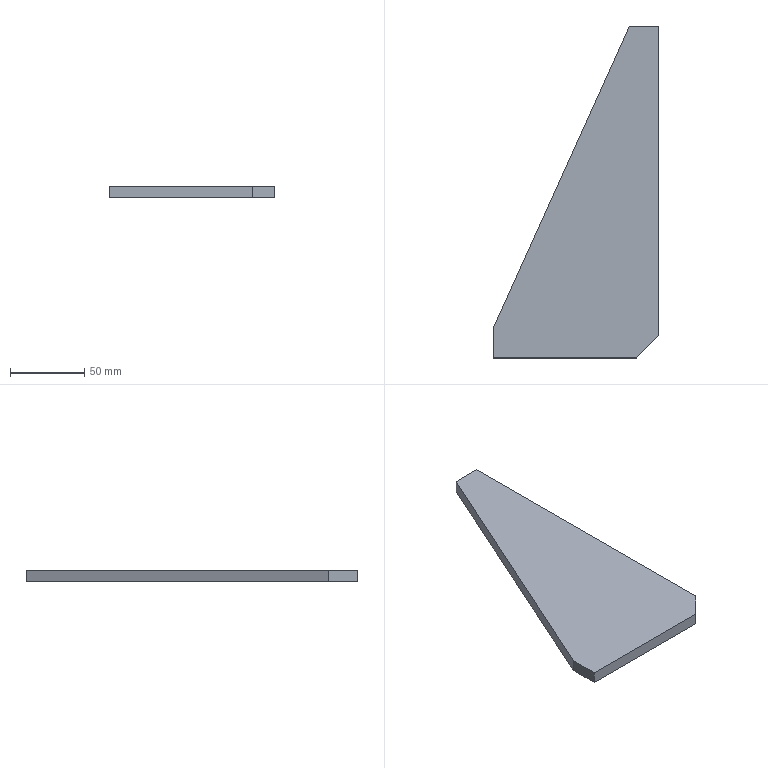Part | STEP file | 02-Rib plate 1 | 1 solid | 8 faces | box 112 x 224 x 8 mm | volume 124732 mm3 | plane 8
STEP:
#1=CARTESIAN_POINT('',(0.,0.,0.));
#2=DIRECTION('',(0.,0.,1.));
#3=DIRECTION('',(1.,0.,0.));
#4=AXIS2_PLACEMENT_3D('',#1,#2,#3);
#5=CARTESIAN_POINT('',(0.,-209.,0.));
#6=VERTEX_POINT('',#5);
#7=CARTESIAN_POINT('',(0.,0.,0.));
#8=VERTEX_POINT('',#7);
#9=CARTESIAN_POINT('',(0.,0.,0.));
#10=DIRECTION('',(0.,1.,0.));
#11=VECTOR('',#10,1.);
#12=LINE('',#9,#11);
#13=CARTESIAN_POINT('',(0.,0.,8.));
#14=DIRECTION('',(-1.,0.,0.));
#15=DIRECTION('',(0.,-1.,0.));
#16=AXIS2_PLACEMENT_3D('',#13,#14,#15);
#17=PLANE('',#16);
#18=CARTESIAN_POINT('',(0.,-8.));
#19=DIRECTION('',(-1.,0.));
#20=VECTOR('',#19,1.);
#21=LINE('',#18,#20);
#22=(GEOMETRIC_REPRESENTATION_CONTEXT(2)PARAMETRIC_REPRESENTATION_CONTEXT()REPRESENTATION_CONTEXT('',''));
#23=DEFINITIONAL_REPRESENTATION('',(#21),#22);
#24=PCURVE('',#17,#23);
#25=CARTESIAN_POINT('',(0.,0.,0.));
#26=DIRECTION('',(0.,0.,-1.));
#27=DIRECTION('',(-1.,0.,0.));
#28=AXIS2_PLACEMENT_3D('',#25,#26,#27);
#29=PLANE('',#28);
#30=CARTESIAN_POINT('',(0.,0.));
#31=DIRECTION('',(0.,1.));
#32=VECTOR('',#31,1.);
#33=LINE('',#30,#32);
#34=(GEOMETRIC_REPRESENTATION_CONTEXT(2)PARAMETRIC_REPRESENTATION_CONTEXT()REPRESENTATION_CONTEXT('',''));
#35=DEFINITIONAL_REPRESENTATION('',(#33),#34);
#36=PCURVE('',#29,#35);
#37=SURFACE_CURVE('',#12,(#24,#36),.PCURVE_S1.);
#38=EDGE_CURVE('',#6,#8,#37,.T.);
#39=ORIENTED_EDGE('',*,*,#38,.T.);
#40=CARTESIAN_POINT('',(0.,0.,8.));
#41=VERTEX_POINT('',#40);
#42=CARTESIAN_POINT('',(0.,0.,8.));
#43=DIRECTION('',(0.,0.,-1.));
#44=VECTOR('',#43,1.);
#45=LINE('',#42,#44);
#46=CARTESIAN_POINT('',(0.,0.));
#47=DIRECTION('',(0.,-1.));
#48=VECTOR('',#47,1.);
#49=LINE('',#46,#48);
#50=(GEOMETRIC_REPRESENTATION_CONTEXT(2)PARAMETRIC_REPRESENTATION_CONTEXT()REPRESENTATION_CONTEXT('',''));
#51=DEFINITIONAL_REPRESENTATION('',(#49),#50);
#52=PCURVE('',#17,#51);
#53=CARTESIAN_POINT('',(0.,0.,8.));
#54=DIRECTION('',(0.,-1.,0.));
#55=DIRECTION('',(1.,0.,0.));
#56=AXIS2_PLACEMENT_3D('',#53,#54,#55);
#57=PLANE('',#56);
#58=CARTESIAN_POINT('',(0.,0.));
#59=DIRECTION('',(0.,-1.));
#60=VECTOR('',#59,1.);
#61=LINE('',#58,#60);
#62=(GEOMETRIC_REPRESENTATION_CONTEXT(2)PARAMETRIC_REPRESENTATION_CONTEXT()REPRESENTATION_CONTEXT('',''));
#63=DEFINITIONAL_REPRESENTATION('',(#61),#62);
#64=PCURVE('',#57,#63);
#65=SURFACE_CURVE('',#45,(#52,#64),.PCURVE_S1.);
#66=EDGE_CURVE('',#41,#8,#65,.T.);
#67=ORIENTED_EDGE('',*,*,#66,.F.);
#68=CARTESIAN_POINT('',(0.,-209.,8.));
#69=VERTEX_POINT('',#68);
#70=CARTESIAN_POINT('',(0.,0.,8.));
#71=DIRECTION('',(0.,1.,0.));
#72=VECTOR('',#71,1.);
#73=LINE('',#70,#72);
#74=CARTESIAN_POINT('',(0.,0.));
#75=DIRECTION('',(-1.,0.));
#76=VECTOR('',#75,1.);
#77=LINE('',#74,#76);
#78=(GEOMETRIC_REPRESENTATION_CONTEXT(2)PARAMETRIC_REPRESENTATION_CONTEXT()REPRESENTATION_CONTEXT('',''));
#79=DEFINITIONAL_REPRESENTATION('',(#77),#78);
#80=PCURVE('',#17,#79);
#81=CARTESIAN_POINT('',(0.,0.,8.));
#82=DIRECTION('',(0.,0.,-1.));
#83=DIRECTION('',(-1.,0.,0.));
#84=AXIS2_PLACEMENT_3D('',#81,#82,#83);
#85=PLANE('',#84);
#86=CARTESIAN_POINT('',(0.,0.));
#87=DIRECTION('',(0.,1.));
#88=VECTOR('',#87,1.);
#89=LINE('',#86,#88);
#90=(GEOMETRIC_REPRESENTATION_CONTEXT(2)PARAMETRIC_REPRESENTATION_CONTEXT()REPRESENTATION_CONTEXT('',''));
#91=DEFINITIONAL_REPRESENTATION('',(#89),#90);
#92=PCURVE('',#85,#91);
#93=SURFACE_CURVE('',#73,(#80,#92),.PCURVE_S1.);
#94=EDGE_CURVE('',#69,#41,#93,.T.);
#95=ORIENTED_EDGE('',*,*,#94,.F.);
#96=CARTESIAN_POINT('',(0.,-209.,8.));
#97=DIRECTION('',(0.,0.,-1.));
#98=VECTOR('',#97,1.);
#99=LINE('',#96,#98);
#100=CARTESIAN_POINT('',(209.,0.));
#101=DIRECTION('',(0.,-1.));
#102=VECTOR('',#101,1.);
#103=LINE('',#100,#102);
#104=(GEOMETRIC_REPRESENTATION_CONTEXT(2)PARAMETRIC_REPRESENTATION_CONTEXT()REPRESENTATION_CONTEXT('',''));
#105=DEFINITIONAL_REPRESENTATION('',(#103),#104);
#106=PCURVE('',#17,#105);
#107=CARTESIAN_POINT('',(0.,-209.,8.));
#108=DIRECTION('',(-0.7071,0.7071,0.));
#109=DIRECTION('',(-0.7071,-0.7071,0.));
#110=AXIS2_PLACEMENT_3D('',#107,#108,#109);
#111=PLANE('',#110);
#112=CARTESIAN_POINT('',(0.,0.));
#113=DIRECTION('',(0.,-1.));
#114=VECTOR('',#113,1.);
#115=LINE('',#112,#114);
#116=(GEOMETRIC_REPRESENTATION_CONTEXT(2)PARAMETRIC_REPRESENTATION_CONTEXT()REPRESENTATION_CONTEXT('',''));
#117=DEFINITIONAL_REPRESENTATION('',(#115),#116);
#118=PCURVE('',#111,#117);
#119=SURFACE_CURVE('',#99,(#106,#118),.PCURVE_S1.);
#120=EDGE_CURVE('',#69,#6,#119,.T.);
#121=ORIENTED_EDGE('',*,*,#120,.T.);
#122=EDGE_LOOP('',(#39,#67,#95,#121));
#123=FACE_BOUND('',#122,.T.);
#124=ADVANCED_FACE('',(#123),#17,.F.);
#125=CARTESIAN_POINT('',(-20.,0.,0.));
#126=VERTEX_POINT('',#125);
#127=CARTESIAN_POINT('',(0.,0.,0.));
#128=DIRECTION('',(-1.,0.,0.));
#129=VECTOR('',#128,1.);
#130=LINE('',#127,#129);
#131=CARTESIAN_POINT('',(0.,-8.));
#132=DIRECTION('',(-1.,0.));
#133=VECTOR('',#132,1.);
#134=LINE('',#131,#133);
#135=(GEOMETRIC_REPRESENTATION_CONTEXT(2)PARAMETRIC_REPRESENTATION_CONTEXT()REPRESENTATION_CONTEXT('',''));
#136=DEFINITIONAL_REPRESENTATION('',(#134),#135);
#137=PCURVE('',#57,#136);
#138=CARTESIAN_POINT('',(0.,0.));
#139=DIRECTION('',(1.,0.));
#140=VECTOR('',#139,1.);
#141=LINE('',#138,#140);
#142=(GEOMETRIC_REPRESENTATION_CONTEXT(2)PARAMETRIC_REPRESENTATION_CONTEXT()REPRESENTATION_CONTEXT('',''));
#143=DEFINITIONAL_REPRESENTATION('',(#141),#142);
#144=PCURVE('',#29,#143);
#145=SURFACE_CURVE('',#130,(#137,#144),.PCURVE_S1.);
#146=EDGE_CURVE('',#8,#126,#145,.T.);
#147=ORIENTED_EDGE('',*,*,#146,.T.);
#148=CARTESIAN_POINT('',(-20.,0.,8.));
#149=VERTEX_POINT('',#148);
#150=CARTESIAN_POINT('',(-20.,0.,8.));
#151=DIRECTION('',(0.,0.,-1.));
#152=VECTOR('',#151,1.);
#153=LINE('',#150,#152);
#154=CARTESIAN_POINT('',(-20.,0.));
#155=DIRECTION('',(0.,-1.));
#156=VECTOR('',#155,1.);
#157=LINE('',#154,#156);
#158=(GEOMETRIC_REPRESENTATION_CONTEXT(2)PARAMETRIC_REPRESENTATION_CONTEXT()REPRESENTATION_CONTEXT('',''));
#159=DEFINITIONAL_REPRESENTATION('',(#157),#158);
#160=PCURVE('',#57,#159);
#161=CARTESIAN_POINT('',(-20.,0.,8.));
#162=DIRECTION('',(0.9116,-0.4111,0.));
#163=DIRECTION('',(0.4111,0.9116,0.));
#164=AXIS2_PLACEMENT_3D('',#161,#162,#163);
#165=PLANE('',#164);
#166=CARTESIAN_POINT('',(0.,0.));
#167=DIRECTION('',(0.,-1.));
#168=VECTOR('',#167,1.);
#169=LINE('',#166,#168);
#170=(GEOMETRIC_REPRESENTATION_CONTEXT(2)PARAMETRIC_REPRESENTATION_CONTEXT()REPRESENTATION_CONTEXT('',''));
#171=DEFINITIONAL_REPRESENTATION('',(#169),#170);
#172=PCURVE('',#165,#171);
#173=SURFACE_CURVE('',#153,(#160,#172),.PCURVE_S1.);
#174=EDGE_CURVE('',#149,#126,#173,.T.);
#175=ORIENTED_EDGE('',*,*,#174,.F.);
#176=CARTESIAN_POINT('',(0.,0.,8.));
#177=DIRECTION('',(-1.,0.,0.));
#178=VECTOR('',#177,1.);
#179=LINE('',#176,#178);
#180=CARTESIAN_POINT('',(0.,0.));
#181=DIRECTION('',(-1.,0.));
#182=VECTOR('',#181,1.);
#183=LINE('',#180,#182);
#184=(GEOMETRIC_REPRESENTATION_CONTEXT(2)PARAMETRIC_REPRESENTATION_CONTEXT()REPRESENTATION_CONTEXT('',''));
#185=DEFINITIONAL_REPRESENTATION('',(#183),#184);
#186=PCURVE('',#57,#185);
#187=CARTESIAN_POINT('',(0.,0.));
#188=DIRECTION('',(1.,0.));
#189=VECTOR('',#188,1.);
#190=LINE('',#187,#189);
#191=(GEOMETRIC_REPRESENTATION_CONTEXT(2)PARAMETRIC_REPRESENTATION_CONTEXT()REPRESENTATION_CONTEXT('',''));
#192=DEFINITIONAL_REPRESENTATION('',(#190),#191);
#193=PCURVE('',#85,#192);
#194=SURFACE_CURVE('',#179,(#186,#193),.PCURVE_S1.);
#195=EDGE_CURVE('',#41,#149,#194,.T.);
#196=ORIENTED_EDGE('',*,*,#195,.F.);
#197=ORIENTED_EDGE('',*,*,#66,.T.);
#198=EDGE_LOOP('',(#147,#175,#196,#197));
#199=FACE_BOUND('',#198,.T.);
#200=ADVANCED_FACE('',(#199),#57,.F.);
#201=CARTESIAN_POINT('',(-112.,-204.,0.));
#202=VERTEX_POINT('',#201);
#203=CARTESIAN_POINT('',(-20.,0.,0.));
#204=DIRECTION('',(-0.4111,-0.9116,0.));
#205=VECTOR('',#204,1.);
#206=LINE('',#203,#205);
#207=CARTESIAN_POINT('',(0.,-8.));
#208=DIRECTION('',(-1.,0.));
#209=VECTOR('',#208,1.);
#210=LINE('',#207,#209);
#211=(GEOMETRIC_REPRESENTATION_CONTEXT(2)PARAMETRIC_REPRESENTATION_CONTEXT()REPRESENTATION_CONTEXT('',''));
#212=DEFINITIONAL_REPRESENTATION('',(#210),#211);
#213=PCURVE('',#165,#212);
#214=CARTESIAN_POINT('',(20.,0.));
#215=DIRECTION('',(0.4111,-0.9116));
#216=VECTOR('',#215,1.);
#217=LINE('',#214,#216);
#218=(GEOMETRIC_REPRESENTATION_CONTEXT(2)PARAMETRIC_REPRESENTATION_CONTEXT()REPRESENTATION_CONTEXT('',''));
#219=DEFINITIONAL_REPRESENTATION('',(#217),#218);
#220=PCURVE('',#29,#219);
#221=SURFACE_CURVE('',#206,(#213,#220),.PCURVE_S1.);
#222=EDGE_CURVE('',#126,#202,#221,.T.);
#223=ORIENTED_EDGE('',*,*,#222,.T.);
#224=CARTESIAN_POINT('',(-112.,-204.,8.));
#225=VERTEX_POINT('',#224);
#226=CARTESIAN_POINT('',(-112.,-204.,8.));
#227=DIRECTION('',(0.,0.,-1.));
#228=VECTOR('',#227,1.);
#229=LINE('',#226,#228);
#230=CARTESIAN_POINT('',(-223.786,0.));
#231=DIRECTION('',(0.,-1.));
#232=VECTOR('',#231,1.);
#233=LINE('',#230,#232);
#234=(GEOMETRIC_REPRESENTATION_CONTEXT(2)PARAMETRIC_REPRESENTATION_CONTEXT()REPRESENTATION_CONTEXT('',''));
#235=DEFINITIONAL_REPRESENTATION('',(#233),#234);
#236=PCURVE('',#165,#235);
#237=CARTESIAN_POINT('',(-112.,-204.,8.));
#238=DIRECTION('',(1.,0.,0.));
#239=DIRECTION('',(0.,1.,0.));
#240=AXIS2_PLACEMENT_3D('',#237,#238,#239);
#241=PLANE('',#240);
#242=CARTESIAN_POINT('',(0.,0.));
#243=DIRECTION('',(0.,-1.));
#244=VECTOR('',#243,1.);
#245=LINE('',#242,#244);
#246=(GEOMETRIC_REPRESENTATION_CONTEXT(2)PARAMETRIC_REPRESENTATION_CONTEXT()REPRESENTATION_CONTEXT('',''));
#247=DEFINITIONAL_REPRESENTATION('',(#245),#246);
#248=PCURVE('',#241,#247);
#249=SURFACE_CURVE('',#229,(#236,#248),.PCURVE_S1.);
#250=EDGE_CURVE('',#225,#202,#249,.T.);
#251=ORIENTED_EDGE('',*,*,#250,.F.);
#252=CARTESIAN_POINT('',(-20.,0.,8.));
#253=DIRECTION('',(-0.4111,-0.9116,0.));
#254=VECTOR('',#253,1.);
#255=LINE('',#252,#254);
#256=CARTESIAN_POINT('',(0.,0.));
#257=DIRECTION('',(-1.,0.));
#258=VECTOR('',#257,1.);
#259=LINE('',#256,#258);
#260=(GEOMETRIC_REPRESENTATION_CONTEXT(2)PARAMETRIC_REPRESENTATION_CONTEXT()REPRESENTATION_CONTEXT('',''));
#261=DEFINITIONAL_REPRESENTATION('',(#259),#260);
#262=PCURVE('',#165,#261);
#263=CARTESIAN_POINT('',(20.,0.));
#264=DIRECTION('',(0.4111,-0.9116));
#265=VECTOR('',#264,1.);
#266=LINE('',#263,#265);
#267=(GEOMETRIC_REPRESENTATION_CONTEXT(2)PARAMETRIC_REPRESENTATION_CONTEXT()REPRESENTATION_CONTEXT('',''));
#268=DEFINITIONAL_REPRESENTATION('',(#266),#267);
#269=PCURVE('',#85,#268);
#270=SURFACE_CURVE('',#255,(#262,#269),.PCURVE_S1.);
#271=EDGE_CURVE('',#149,#225,#270,.T.);
#272=ORIENTED_EDGE('',*,*,#271,.F.);
#273=ORIENTED_EDGE('',*,*,#174,.T.);
#274=EDGE_LOOP('',(#223,#251,#272,#273));
#275=FACE_BOUND('',#274,.T.);
#276=ADVANCED_FACE('',(#275),#165,.F.);
#277=CARTESIAN_POINT('',(-112.,-224.,0.));
#278=VERTEX_POINT('',#277);
#279=CARTESIAN_POINT('',(-112.,-204.,0.));
#280=DIRECTION('',(0.,-1.,0.));
#281=VECTOR('',#280,1.);
#282=LINE('',#279,#281);
#283=CARTESIAN_POINT('',(0.,-8.));
#284=DIRECTION('',(-1.,0.));
#285=VECTOR('',#284,1.);
#286=LINE('',#283,#285);
#287=(GEOMETRIC_REPRESENTATION_CONTEXT(2)PARAMETRIC_REPRESENTATION_CONTEXT()REPRESENTATION_CONTEXT('',''));
#288=DEFINITIONAL_REPRESENTATION('',(#286),#287);
#289=PCURVE('',#241,#288);
#290=CARTESIAN_POINT('',(112.,-204.));
#291=DIRECTION('',(0.,-1.));
#292=VECTOR('',#291,1.);
#293=LINE('',#290,#292);
#294=(GEOMETRIC_REPRESENTATION_CONTEXT(2)PARAMETRIC_REPRESENTATION_CONTEXT()REPRESENTATION_CONTEXT('',''));
#295=DEFINITIONAL_REPRESENTATION('',(#293),#294);
#296=PCURVE('',#29,#295);
#297=SURFACE_CURVE('',#282,(#289,#296),.PCURVE_S1.);
#298=EDGE_CURVE('',#202,#278,#297,.T.);
#299=ORIENTED_EDGE('',*,*,#298,.T.);
#300=CARTESIAN_POINT('',(-112.,-224.,8.));
#301=VERTEX_POINT('',#300);
#302=CARTESIAN_POINT('',(-112.,-224.,8.));
#303=DIRECTION('',(0.,0.,-1.));
#304=VECTOR('',#303,1.);
#305=LINE('',#302,#304);
#306=CARTESIAN_POINT('',(-20.,0.));
#307=DIRECTION('',(0.,-1.));
#308=VECTOR('',#307,1.);
#309=LINE('',#306,#308);
#310=(GEOMETRIC_REPRESENTATION_CONTEXT(2)PARAMETRIC_REPRESENTATION_CONTEXT()REPRESENTATION_CONTEXT('',''));
#311=DEFINITIONAL_REPRESENTATION('',(#309),#310);
#312=PCURVE('',#241,#311);
#313=CARTESIAN_POINT('',(-15.,-224.,8.));
#314=DIRECTION('',(0.,1.,0.));
#315=DIRECTION('',(0.,0.,1.));
#316=AXIS2_PLACEMENT_3D('',#313,#314,#315);
#317=PLANE('',#316);
#318=CARTESIAN_POINT('',(0.,-97.));
#319=DIRECTION('',(-1.,0.));
#320=VECTOR('',#319,1.);
#321=LINE('',#318,#320);
#322=(GEOMETRIC_REPRESENTATION_CONTEXT(2)PARAMETRIC_REPRESENTATION_CONTEXT()REPRESENTATION_CONTEXT('',''));
#323=DEFINITIONAL_REPRESENTATION('',(#321),#322);
#324=PCURVE('',#317,#323);
#325=SURFACE_CURVE('',#305,(#312,#324),.PCURVE_S1.);
#326=EDGE_CURVE('',#301,#278,#325,.T.);
#327=ORIENTED_EDGE('',*,*,#326,.F.);
#328=CARTESIAN_POINT('',(-112.,-204.,8.));
#329=DIRECTION('',(0.,-1.,0.));
#330=VECTOR('',#329,1.);
#331=LINE('',#328,#330);
#332=CARTESIAN_POINT('',(0.,0.));
#333=DIRECTION('',(-1.,0.));
#334=VECTOR('',#333,1.);
#335=LINE('',#332,#334);
#336=(GEOMETRIC_REPRESENTATION_CONTEXT(2)PARAMETRIC_REPRESENTATION_CONTEXT()REPRESENTATION_CONTEXT('',''));
#337=DEFINITIONAL_REPRESENTATION('',(#335),#336);
#338=PCURVE('',#241,#337);
#339=CARTESIAN_POINT('',(112.,-204.));
#340=DIRECTION('',(0.,-1.));
#341=VECTOR('',#340,1.);
#342=LINE('',#339,#341);
#343=(GEOMETRIC_REPRESENTATION_CONTEXT(2)PARAMETRIC_REPRESENTATION_CONTEXT()REPRESENTATION_CONTEXT('',''));
#344=DEFINITIONAL_REPRESENTATION('',(#342),#343);
#345=PCURVE('',#85,#344);
#346=SURFACE_CURVE('',#331,(#338,#345),.PCURVE_S1.);
#347=EDGE_CURVE('',#225,#301,#346,.T.);
#348=ORIENTED_EDGE('',*,*,#347,.F.);
#349=ORIENTED_EDGE('',*,*,#250,.T.);
#350=EDGE_LOOP('',(#299,#327,#348,#349));
#351=FACE_BOUND('',#350,.T.);
#352=ADVANCED_FACE('',(#351),#241,.F.);
#353=CARTESIAN_POINT('',(-15.,-224.,0.));
#354=VERTEX_POINT('',#353);
#355=CARTESIAN_POINT('',(-15.,-224.,0.));
#356=DIRECTION('',(1.,0.,0.));
#357=VECTOR('',#356,1.);
#358=LINE('',#355,#357);
#359=CARTESIAN_POINT('',(-8.,0.));
#360=DIRECTION('',(0.,1.));
#361=VECTOR('',#360,1.);
#362=LINE('',#359,#361);
#363=(GEOMETRIC_REPRESENTATION_CONTEXT(2)PARAMETRIC_REPRESENTATION_CONTEXT()REPRESENTATION_CONTEXT('',''));
#364=DEFINITIONAL_REPRESENTATION('',(#362),#363);
#365=PCURVE('',#317,#364);
#366=CARTESIAN_POINT('',(15.,-224.));
#367=DIRECTION('',(-1.,0.));
#368=VECTOR('',#367,1.);
#369=LINE('',#366,#368);
#370=(GEOMETRIC_REPRESENTATION_CONTEXT(2)PARAMETRIC_REPRESENTATION_CONTEXT()REPRESENTATION_CONTEXT('',''));
#371=DEFINITIONAL_REPRESENTATION('',(#369),#370);
#372=PCURVE('',#29,#371);
#373=SURFACE_CURVE('',#358,(#365,#372),.PCURVE_S1.);
#374=EDGE_CURVE('',#278,#354,#373,.T.);
#375=ORIENTED_EDGE('',*,*,#374,.T.);
#376=CARTESIAN_POINT('',(-15.,-224.,8.));
#377=VERTEX_POINT('',#376);
#378=CARTESIAN_POINT('',(-15.,-224.,8.));
#379=DIRECTION('',(0.,0.,-1.));
#380=VECTOR('',#379,1.);
#381=LINE('',#378,#380);
#382=CARTESIAN_POINT('',(0.,0.));
#383=DIRECTION('',(-1.,0.));
#384=VECTOR('',#383,1.);
#385=LINE('',#382,#384);
#386=(GEOMETRIC_REPRESENTATION_CONTEXT(2)PARAMETRIC_REPRESENTATION_CONTEXT()REPRESENTATION_CONTEXT('',''));
#387=DEFINITIONAL_REPRESENTATION('',(#385),#386);
#388=PCURVE('',#317,#387);
#389=CARTESIAN_POINT('',(21.213,0.));
#390=DIRECTION('',(0.,-1.));
#391=VECTOR('',#390,1.);
#392=LINE('',#389,#391);
#393=(GEOMETRIC_REPRESENTATION_CONTEXT(2)PARAMETRIC_REPRESENTATION_CONTEXT()REPRESENTATION_CONTEXT('',''));
#394=DEFINITIONAL_REPRESENTATION('',(#392),#393);
#395=PCURVE('',#111,#394);
#396=SURFACE_CURVE('',#381,(#388,#395),.PCURVE_S1.);
#397=EDGE_CURVE('',#377,#354,#396,.T.);
#398=ORIENTED_EDGE('',*,*,#397,.F.);
#399=CARTESIAN_POINT('',(-15.,-224.,8.));
#400=DIRECTION('',(1.,0.,0.));
#401=VECTOR('',#400,1.);
#402=LINE('',#399,#401);
#403=CARTESIAN_POINT('',(0.,0.));
#404=DIRECTION('',(0.,1.));
#405=VECTOR('',#404,1.);
#406=LINE('',#403,#405);
#407=(GEOMETRIC_REPRESENTATION_CONTEXT(2)PARAMETRIC_REPRESENTATION_CONTEXT()REPRESENTATION_CONTEXT('',''));
#408=DEFINITIONAL_REPRESENTATION('',(#406),#407);
#409=PCURVE('',#317,#408);
#410=CARTESIAN_POINT('',(15.,-224.));
#411=DIRECTION('',(-1.,0.));
#412=VECTOR('',#411,1.);
#413=LINE('',#410,#412);
#414=(GEOMETRIC_REPRESENTATION_CONTEXT(2)PARAMETRIC_REPRESENTATION_CONTEXT()REPRESENTATION_CONTEXT('',''));
#415=DEFINITIONAL_REPRESENTATION('',(#413),#414);
#416=PCURVE('',#85,#415);
#417=SURFACE_CURVE('',#402,(#409,#416),.PCURVE_S1.);
#418=EDGE_CURVE('',#301,#377,#417,.T.);
#419=ORIENTED_EDGE('',*,*,#418,.F.);
#420=ORIENTED_EDGE('',*,*,#326,.T.);
#421=EDGE_LOOP('',(#375,#398,#419,#420));
#422=FACE_BOUND('',#421,.T.);
#423=ADVANCED_FACE('',(#422),#317,.F.);
#424=CARTESIAN_POINT('',(0.,-209.,0.));
#425=DIRECTION('',(0.7071,0.7071,0.));
#426=VECTOR('',#425,1.);
#427=LINE('',#424,#426);
#428=CARTESIAN_POINT('',(0.,-8.));
#429=DIRECTION('',(-1.,0.));
#430=VECTOR('',#429,1.);
#431=LINE('',#428,#430);
#432=(GEOMETRIC_REPRESENTATION_CONTEXT(2)PARAMETRIC_REPRESENTATION_CONTEXT()REPRESENTATION_CONTEXT('',''));
#433=DEFINITIONAL_REPRESENTATION('',(#431),#432);
#434=PCURVE('',#111,#433);
#435=CARTESIAN_POINT('',(0.,-209.));
#436=DIRECTION('',(-0.7071,0.7071));
#437=VECTOR('',#436,1.);
#438=LINE('',#435,#437);
#439=(GEOMETRIC_REPRESENTATION_CONTEXT(2)PARAMETRIC_REPRESENTATION_CONTEXT()REPRESENTATION_CONTEXT('',''));
#440=DEFINITIONAL_REPRESENTATION('',(#438),#439);
#441=PCURVE('',#29,#440);
#442=SURFACE_CURVE('',#427,(#434,#441),.PCURVE_S1.);
#443=EDGE_CURVE('',#354,#6,#442,.T.);
#444=ORIENTED_EDGE('',*,*,#443,.T.);
#445=ORIENTED_EDGE('',*,*,#120,.F.);
#446=CARTESIAN_POINT('',(0.,-209.,8.));
#447=DIRECTION('',(0.7071,0.7071,0.));
#448=VECTOR('',#447,1.);
#449=LINE('',#446,#448);
#450=CARTESIAN_POINT('',(0.,0.));
#451=DIRECTION('',(-1.,0.));
#452=VECTOR('',#451,1.);
#453=LINE('',#450,#452);
#454=(GEOMETRIC_REPRESENTATION_CONTEXT(2)PARAMETRIC_REPRESENTATION_CONTEXT()REPRESENTATION_CONTEXT('',''));
#455=DEFINITIONAL_REPRESENTATION('',(#453),#454);
#456=PCURVE('',#111,#455);
#457=CARTESIAN_POINT('',(0.,-209.));
#458=DIRECTION('',(-0.7071,0.7071));
#459=VECTOR('',#458,1.);
#460=LINE('',#457,#459);
#461=(GEOMETRIC_REPRESENTATION_CONTEXT(2)PARAMETRIC_REPRESENTATION_CONTEXT()REPRESENTATION_CONTEXT('',''));
#462=DEFINITIONAL_REPRESENTATION('',(#460),#461);
#463=PCURVE('',#85,#462);
#464=SURFACE_CURVE('',#449,(#456,#463),.PCURVE_S1.);
#465=EDGE_CURVE('',#377,#69,#464,.T.);
#466=ORIENTED_EDGE('',*,*,#465,.F.);
#467=ORIENTED_EDGE('',*,*,#397,.T.);
#468=EDGE_LOOP('',(#444,#445,#466,#467));
#469=FACE_BOUND('',#468,.T.);
#470=ADVANCED_FACE('',(#469),#111,.F.);
#471=ORIENTED_EDGE('',*,*,#94,.T.);
#472=ORIENTED_EDGE('',*,*,#195,.T.);
#473=ORIENTED_EDGE('',*,*,#271,.T.);
#474=ORIENTED_EDGE('',*,*,#347,.T.);
#475=ORIENTED_EDGE('',*,*,#418,.T.);
#476=ORIENTED_EDGE('',*,*,#465,.T.);
#477=EDGE_LOOP('',(#471,#472,#473,#474,#475,#476));
#478=FACE_BOUND('',#477,.T.);
#479=ADVANCED_FACE('',(#478),#85,.F.);
#480=ORIENTED_EDGE('',*,*,#38,.F.);
#481=ORIENTED_EDGE('',*,*,#443,.F.);
#482=ORIENTED_EDGE('',*,*,#374,.F.);
#483=ORIENTED_EDGE('',*,*,#298,.F.);
#484=ORIENTED_EDGE('',*,*,#222,.F.);
#485=ORIENTED_EDGE('',*,*,#146,.F.);
#486=EDGE_LOOP('',(#480,#481,#482,#483,#484,#485));
#487=FACE_BOUND('',#486,.T.);
#488=ADVANCED_FACE('',(#487),#29,.T.);
#489=CLOSED_SHELL('',(#124,#200,#276,#352,#423,#470,#479,#488));
#490=MANIFOLD_SOLID_BREP('',#489);
#491=(LENGTH_UNIT()NAMED_UNIT(*)SI_UNIT(.MILLI.,.METRE.));
#492=UNCERTAINTY_MEASURE_WITH_UNIT(LENGTH_MEASURE(0.0000001),#491,'','');
#493=(NAMED_UNIT(*)PLANE_ANGLE_UNIT()SI_UNIT($,.RADIAN.));
#494=(NAMED_UNIT(*)SI_UNIT($,.STERADIAN.)SOLID_ANGLE_UNIT());
#495=(GEOMETRIC_REPRESENTATION_CONTEXT(3)GLOBAL_UNCERTAINTY_ASSIGNED_CONTEXT((#492))GLOBAL_UNIT_ASSIGNED_CONTEXT((#491,#493,#494))REPRESENTATION_CONTEXT('',''));
#496=ADVANCED_BREP_SHAPE_REPRESENTATION('',(#4,#490),#495);